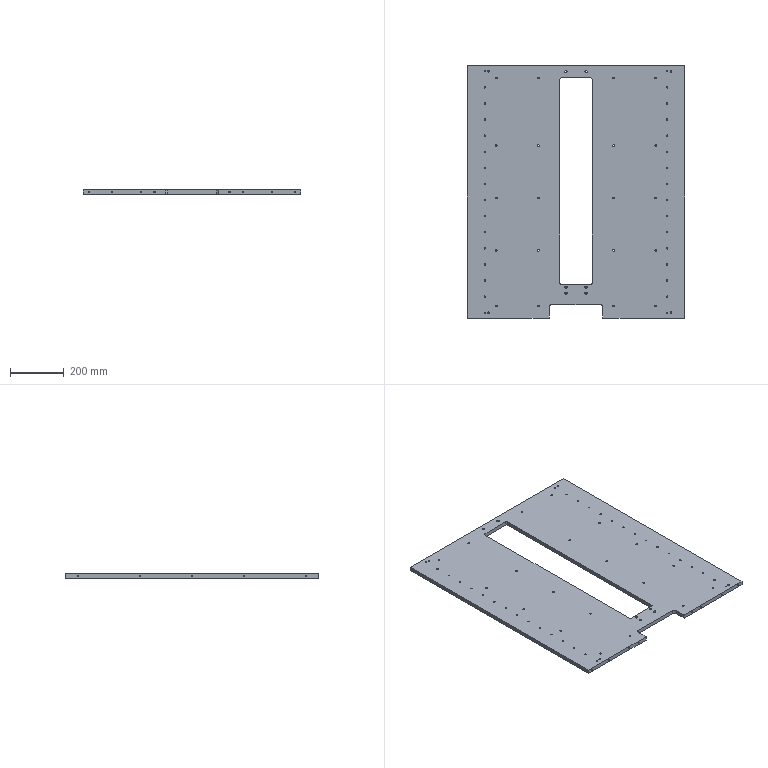Part | STEP file | 0244_202_Plate | 1 solid | 296 faces | box 810 x 940 x 15 mm | volume 9838794 mm3 | cylinder 216 | cone 46 | plane 34 | commonest cylinder face diameters 5 x110 6.6 x40 11 x40 8.5 x12 6 x8 10 x4